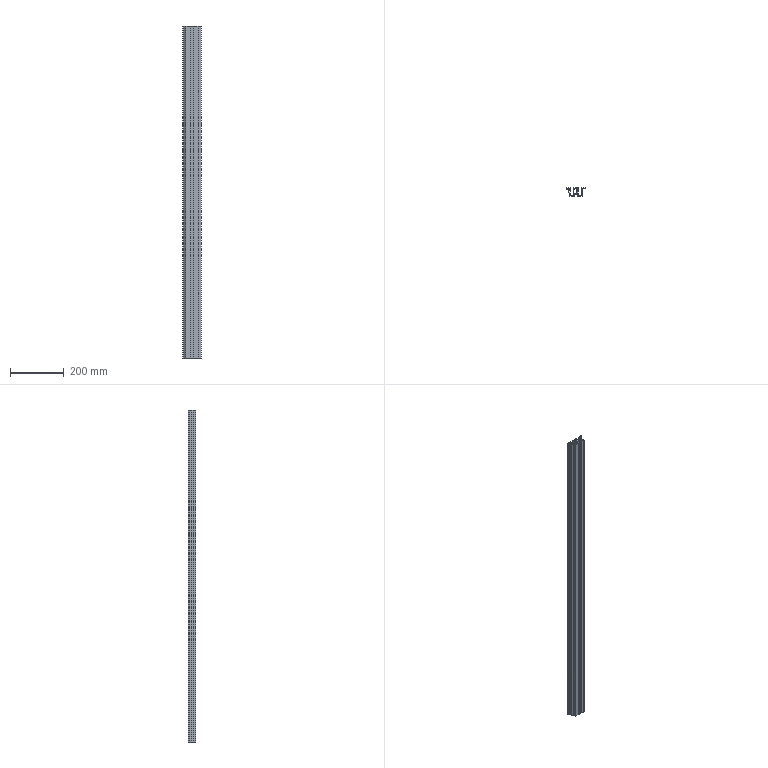Part | SolidWorks | features Emboss 1, Extrusion 1, ICE 1 | 1 solid | 72 faces | box 70 x 29.5 x 1235 mm | volume 447688 mm3 | plane 60 | cylinder 12 | commonest cylinder face diameters 2 x9 3 x3